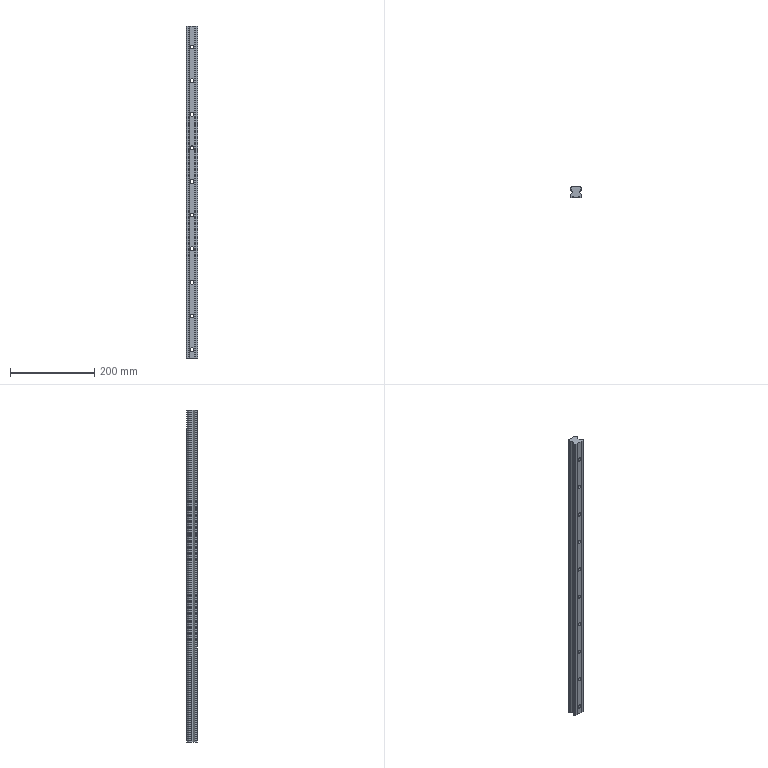Part | STEP file | HGR30_1 | 1 solid | 106 faces | box 28 x 26 x 790 mm | volume 457058 mm3 | cylinder 62 | plane 44 | commonest cylinder face diameters 9 x20 14 x20 1.2 x12 1.6 x6 5.66 x4